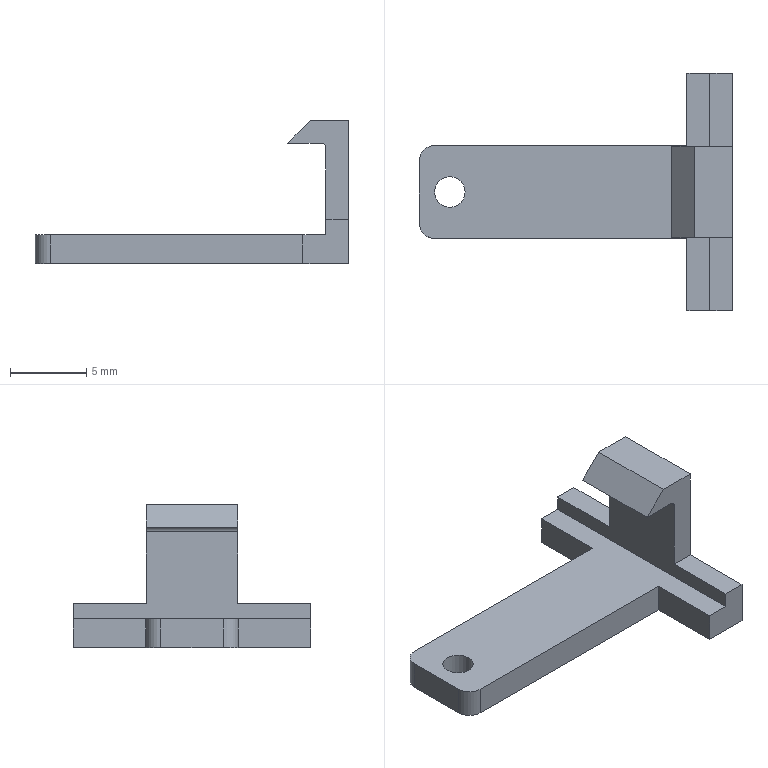Part | NX | features BREP 2, REPLACE_FACE 1, UNITE 1 | 1 solid | 22 faces | box 20.555 x 15.6 x 9.4 mm | volume 383.369 mm3 | plane 18 | cylinder 4 | commonest cylinder face diameters 2 x3 0.6 x1
STEP:
#1=CARTESIAN_POINT('',(-22.19,-197.607,1.));
#2=VERTEX_POINT('',#1);
#3=CARTESIAN_POINT('',(-23.19,-197.607,1.));
#4=DIRECTION('',(0.,0.,1.));
#5=DIRECTION('',(1.,0.,0.));
#6=AXIS2_PLACEMENT_3D('',#3,#4,#5);
#7=CIRCLE('',#6,1.);
#8=EDGE_CURVE('',#2,#2,#7,.T.);
#9=ORIENTED_EDGE('',*,*,#8,.T.);
#10=EDGE_LOOP('',(#9));
#11=FACE_BOUND('',#10,.T.);
#12=CARTESIAN_POINT('',(-22.19,-197.607,-0.9));
#13=VERTEX_POINT('',#12);
#14=CARTESIAN_POINT('',(-23.19,-197.607,-0.9));
#15=DIRECTION('',(0.,0.,1.));
#16=DIRECTION('',(1.,0.,0.));
#17=AXIS2_PLACEMENT_3D('',#14,#15,#16);
#18=CIRCLE('',#17,1.);
#19=EDGE_CURVE('',#13,#13,#18,.T.);
#20=ORIENTED_EDGE('',*,*,#19,.F.);
#21=EDGE_LOOP('',(#20));
#22=FACE_BOUND('',#21,.T.);
#23=CARTESIAN_POINT('',(-23.19,-197.607,-9.));
#24=DIRECTION('',(0.,0.,1.));
#25=DIRECTION('',(-1.,0.,0.));
#26=AXIS2_PLACEMENT_3D('',#23,#24,#25);
#27=CYLINDRICAL_SURFACE('',#26,1.);
#28=ADVANCED_FACE('',(#11,#22),#27,.F.);
#29=CARTESIAN_POINT('',(-4.635,-189.807,2.));
#30=VERTEX_POINT('',#29);
#31=CARTESIAN_POINT('',(-6.135,-189.807,2.));
#32=VERTEX_POINT('',#31);
#33=CARTESIAN_POINT('',(0.,-189.807,2.));
#34=DIRECTION('',(-1.,0.,0.));
#35=VECTOR('',#34,1000.);
#36=LINE('',#33,#35);
#37=EDGE_CURVE('',#30,#32,#36,.T.);
#38=ORIENTED_EDGE('',*,*,#37,.T.);
#39=CARTESIAN_POINT('',(-6.135,-194.607,2.));
#40=VERTEX_POINT('',#39);
#41=CARTESIAN_POINT('',(-6.135,-184.759,2.));
#42=DIRECTION('',(0.,1.,0.));
#43=VECTOR('',#42,1000.);
#44=LINE('',#41,#43);
#45=EDGE_CURVE('',#40,#32,#44,.T.);
#46=ORIENTED_EDGE('',*,*,#45,.F.);
#47=CARTESIAN_POINT('',(-4.635,-194.607,2.));
#48=VERTEX_POINT('',#47);
#49=CARTESIAN_POINT('',(-28.167,-194.607,2.));
#50=DIRECTION('',(1.,0.,0.));
#51=VECTOR('',#50,1000.);
#52=LINE('',#49,#51);
#53=EDGE_CURVE('',#40,#48,#52,.T.);
#54=ORIENTED_EDGE('',*,*,#53,.T.);
#55=CARTESIAN_POINT('',(-4.635,-200.607,2.));
#56=DIRECTION('',(0.,1.,0.));
#57=VECTOR('',#56,1000.);
#58=LINE('',#55,#57);
#59=EDGE_CURVE('',#48,#30,#58,.T.);
#60=ORIENTED_EDGE('',*,*,#59,.T.);
#61=EDGE_LOOP('',(#38,#46,#54,#60));
#62=FACE_BOUND('',#61,.T.);
#63=CARTESIAN_POINT('',(0.,0.,2.));
#64=DIRECTION('',(0.,0.,1.));
#65=DIRECTION('',(-1.,0.,0.));
#66=AXIS2_PLACEMENT_3D('',#63,#64,#65);
#67=PLANE('',#66);
#68=ADVANCED_FACE('',(#62),#67,.T.);
#69=CARTESIAN_POINT('',(-6.135,-200.607,2.));
#70=VERTEX_POINT('',#69);
#71=CARTESIAN_POINT('',(-6.135,-205.407,2.));
#72=VERTEX_POINT('',#71);
#73=CARTESIAN_POINT('',(-6.135,0.,2.));
#74=DIRECTION('',(0.,-1.,0.));
#75=VECTOR('',#74,1000.);
#76=LINE('',#73,#75);
#77=EDGE_CURVE('',#70,#72,#76,.T.);
#78=ORIENTED_EDGE('',*,*,#77,.T.);
#79=CARTESIAN_POINT('',(-4.635,-205.407,2.));
#80=VERTEX_POINT('',#79);
#81=CARTESIAN_POINT('',(0.,-205.407,2.));
#82=DIRECTION('',(1.,0.,0.));
#83=VECTOR('',#82,1000.);
#84=LINE('',#81,#83);
#85=EDGE_CURVE('',#72,#80,#84,.T.);
#86=ORIENTED_EDGE('',*,*,#85,.T.);
#87=CARTESIAN_POINT('',(-4.635,-200.607,2.));
#88=VERTEX_POINT('',#87);
#89=CARTESIAN_POINT('',(-4.635,-200.607,2.));
#90=DIRECTION('',(0.,1.,0.));
#91=VECTOR('',#90,1000.);
#92=LINE('',#89,#91);
#93=EDGE_CURVE('',#80,#88,#92,.T.);
#94=ORIENTED_EDGE('',*,*,#93,.T.);
#95=CARTESIAN_POINT('',(-28.167,-200.607,2.));
#96=DIRECTION('',(-1.,0.,0.));
#97=VECTOR('',#96,1000.);
#98=LINE('',#95,#97);
#99=EDGE_CURVE('',#88,#70,#98,.T.);
#100=ORIENTED_EDGE('',*,*,#99,.T.);
#101=EDGE_LOOP('',(#78,#86,#94,#100));
#102=FACE_BOUND('',#101,.T.);
#103=CARTESIAN_POINT('',(0.,0.,2.));
#104=DIRECTION('',(0.,0.,1.));
#105=DIRECTION('',(-1.,0.,0.));
#106=AXIS2_PLACEMENT_3D('',#103,#104,#105);
#107=PLANE('',#106);
#108=ADVANCED_FACE('',(#102),#107,.T.);
#109=ORIENTED_EDGE('',*,*,#85,.F.);
#110=CARTESIAN_POINT('',(-6.135,-205.407,1.));
#111=VERTEX_POINT('',#110);
#112=CARTESIAN_POINT('',(-6.135,-205.407,0.));
#113=DIRECTION('',(0.,0.,-1.));
#114=VECTOR('',#113,1000.);
#115=LINE('',#112,#114);
#116=EDGE_CURVE('',#72,#111,#115,.T.);
#117=ORIENTED_EDGE('',*,*,#116,.T.);
#118=CARTESIAN_POINT('',(-7.635,-205.407,1.));
#119=VERTEX_POINT('',#118);
#120=CARTESIAN_POINT('',(-4.635,-205.407,1.));
#121=DIRECTION('',(-1.,0.,0.));
#122=VECTOR('',#121,1000.);
#123=LINE('',#120,#122);
#124=EDGE_CURVE('',#111,#119,#123,.T.);
#125=ORIENTED_EDGE('',*,*,#124,.T.);
#126=CARTESIAN_POINT('',(-7.635,-205.407,-0.9));
#127=VERTEX_POINT('',#126);
#128=CARTESIAN_POINT('',(-7.635,-205.407,0.));
#129=DIRECTION('',(0.,0.,1.));
#130=VECTOR('',#129,1000.);
#131=LINE('',#128,#130);
#132=EDGE_CURVE('',#127,#119,#131,.T.);
#133=ORIENTED_EDGE('',*,*,#132,.F.);
#134=CARTESIAN_POINT('',(-4.635,-205.407,-0.9));
#135=VERTEX_POINT('',#134);
#136=CARTESIAN_POINT('',(0.,-205.407,-0.9));
#137=DIRECTION('',(1.,0.,0.));
#138=VECTOR('',#137,1000.);
#139=LINE('',#136,#138);
#140=EDGE_CURVE('',#127,#135,#139,.T.);
#141=ORIENTED_EDGE('',*,*,#140,.T.);
#142=CARTESIAN_POINT('',(-4.635,-205.407,2.));
#143=DIRECTION('',(0.,0.,1.));
#144=VECTOR('',#143,1000.);
#145=LINE('',#142,#144);
#146=EDGE_CURVE('',#135,#80,#145,.T.);
#147=ORIENTED_EDGE('',*,*,#146,.T.);
#148=EDGE_LOOP('',(#109,#117,#125,#133,#141,#147));
#149=FACE_BOUND('',#148,.T.);
#150=CARTESIAN_POINT('',(-4.635,-205.407,0.));
#151=DIRECTION('',(0.,-1.,0.));
#152=DIRECTION('',(0.,0.,1.));
#153=AXIS2_PLACEMENT_3D('',#150,#151,#152);
#154=PLANE('',#153);
#155=ADVANCED_FACE('',(#149),#154,.T.);
#156=ORIENTED_EDGE('',*,*,#132,.T.);
#157=CARTESIAN_POINT('',(-7.635,-200.657,1.));
#158=VERTEX_POINT('',#157);
#159=CARTESIAN_POINT('',(-7.635,0.,1.));
#160=DIRECTION('',(0.,-1.,0.));
#161=VECTOR('',#160,1000.);
#162=LINE('',#159,#161);
#163=EDGE_CURVE('',#158,#119,#162,.T.);
#164=ORIENTED_EDGE('',*,*,#163,.F.);
#165=CARTESIAN_POINT('',(-7.635,-200.657,-0.9));
#166=VERTEX_POINT('',#165);
#167=CARTESIAN_POINT('',(-7.635,-200.657,2.));
#168=DIRECTION('',(0.,0.,1.));
#169=VECTOR('',#168,1000.);
#170=LINE('',#167,#169);
#171=EDGE_CURVE('',#166,#158,#170,.T.);
#172=ORIENTED_EDGE('',*,*,#171,.F.);
#173=CARTESIAN_POINT('',(-7.635,0.,-0.9));
#174=DIRECTION('',(0.,-1.,0.));
#175=VECTOR('',#174,1000.);
#176=LINE('',#173,#175);
#177=EDGE_CURVE('',#166,#127,#176,.T.);
#178=ORIENTED_EDGE('',*,*,#177,.T.);
#179=EDGE_LOOP('',(#156,#164,#172,#178));
#180=FACE_BOUND('',#179,.T.);
#181=CARTESIAN_POINT('',(-7.635,-203.607,0.));
#182=DIRECTION('',(-1.,0.,0.));
#183=DIRECTION('',(0.,-1.,0.));
#184=AXIS2_PLACEMENT_3D('',#181,#182,#183);
#185=PLANE('',#184);
#186=ADVANCED_FACE('',(#180),#185,.T.);
#187=CARTESIAN_POINT('',(-7.635,-194.557,1.));
#188=VERTEX_POINT('',#187);
#189=CARTESIAN_POINT('',(-7.635,-189.807,1.));
#190=VERTEX_POINT('',#189);
#191=CARTESIAN_POINT('',(-7.635,-191.607,1.));
#192=DIRECTION('',(0.,1.,0.));
#193=VECTOR('',#192,1000.);
#194=LINE('',#191,#193);
#195=EDGE_CURVE('',#188,#190,#194,.T.);
#196=ORIENTED_EDGE('',*,*,#195,.T.);
#197=CARTESIAN_POINT('',(-7.635,-189.807,-0.9));
#198=VERTEX_POINT('',#197);
#199=CARTESIAN_POINT('',(-7.635,-189.807,0.));
#200=DIRECTION('',(0.,0.,1.));
#201=VECTOR('',#200,1000.);
#202=LINE('',#199,#201);
#203=EDGE_CURVE('',#198,#190,#202,.T.);
#204=ORIENTED_EDGE('',*,*,#203,.F.);
#205=CARTESIAN_POINT('',(-7.635,-194.557,-0.9));
#206=VERTEX_POINT('',#205);
#207=CARTESIAN_POINT('',(-7.635,0.,-0.9));
#208=DIRECTION('',(0.,-1.,0.));
#209=VECTOR('',#208,1000.);
#210=LINE('',#207,#209);
#211=EDGE_CURVE('',#198,#206,#210,.T.);
#212=ORIENTED_EDGE('',*,*,#211,.T.);
#213=CARTESIAN_POINT('',(-7.635,-194.557,0.));
#214=DIRECTION('',(0.,0.,1.));
#215=VECTOR('',#214,1000.);
#216=LINE('',#213,#215);
#217=EDGE_CURVE('',#206,#188,#216,.T.);
#218=ORIENTED_EDGE('',*,*,#217,.T.);
#219=EDGE_LOOP('',(#196,#204,#212,#218));
#220=FACE_BOUND('',#219,.T.);
#221=CARTESIAN_POINT('',(-7.635,-191.607,0.));
#222=DIRECTION('',(-1.,0.,0.));
#223=DIRECTION('',(0.,0.,-1.));
#224=AXIS2_PLACEMENT_3D('',#221,#222,#223);
#225=PLANE('',#224);
#226=ADVANCED_FACE('',(#220),#225,.T.);
#227=CARTESIAN_POINT('',(-6.135,-189.807,1.));
#228=VERTEX_POINT('',#227);
#229=CARTESIAN_POINT('',(-4.635,-189.807,1.));
#230=DIRECTION('',(1.,0.,0.));
#231=VECTOR('',#230,1000.);
#232=LINE('',#229,#231);
#233=EDGE_CURVE('',#190,#228,#232,.T.);
#234=ORIENTED_EDGE('',*,*,#233,.T.);
#235=CARTESIAN_POINT('',(-6.135,-189.807,0.));
#236=DIRECTION('',(0.,0.,1.));
#237=VECTOR('',#236,1000.);
#238=LINE('',#235,#237);
#239=EDGE_CURVE('',#228,#32,#238,.T.);
#240=ORIENTED_EDGE('',*,*,#239,.T.);
#241=ORIENTED_EDGE('',*,*,#37,.F.);
#242=CARTESIAN_POINT('',(-4.635,-189.807,-0.9));
#243=VERTEX_POINT('',#242);
#244=CARTESIAN_POINT('',(-4.635,-189.807,0.));
#245=DIRECTION('',(0.,0.,1.));
#246=VECTOR('',#245,1000.);
#247=LINE('',#244,#246);
#248=EDGE_CURVE('',#243,#30,#247,.T.);
#249=ORIENTED_EDGE('',*,*,#248,.F.);
#250=CARTESIAN_POINT('',(0.,-189.807,-0.9));
#251=DIRECTION('',(-1.,0.,0.));
#252=VECTOR('',#251,1000.);
#253=LINE('',#250,#252);
#254=EDGE_CURVE('',#243,#198,#253,.T.);
#255=ORIENTED_EDGE('',*,*,#254,.T.);
#256=ORIENTED_EDGE('',*,*,#203,.T.);
#257=EDGE_LOOP('',(#234,#240,#241,#249,#255,#256));
#258=FACE_BOUND('',#257,.T.);
#259=CARTESIAN_POINT('',(-4.635,-189.807,0.));
#260=DIRECTION('',(0.,1.,0.));
#261=DIRECTION('',(-1.,0.,0.));
#262=AXIS2_PLACEMENT_3D('',#259,#260,#261);
#263=PLANE('',#262);
#264=ADVANCED_FACE('',(#258),#263,.T.);
#265=CARTESIAN_POINT('',(-24.19,-194.557,-0.9));
#266=VERTEX_POINT('',#265);
#267=CARTESIAN_POINT('',(-4.635,-194.557,-0.9));
#268=DIRECTION('',(-1.,0.,0.));
#269=VECTOR('',#268,1000.);
#270=LINE('',#267,#269);
#271=EDGE_CURVE('',#206,#266,#270,.T.);
#272=ORIENTED_EDGE('',*,*,#271,.T.);
#273=CARTESIAN_POINT('',(-24.19,-194.557,1.));
#274=VERTEX_POINT('',#273);
#275=CARTESIAN_POINT('',(-24.19,-194.557,2.));
#276=DIRECTION('',(0.,0.,1.));
#277=VECTOR('',#276,1000.);
#278=LINE('',#275,#277);
#279=EDGE_CURVE('',#266,#274,#278,.T.);
#280=ORIENTED_EDGE('',*,*,#279,.T.);
#281=CARTESIAN_POINT('',(-4.635,-194.557,1.));
#282=DIRECTION('',(-1.,0.,0.));
#283=VECTOR('',#282,1000.);
#284=LINE('',#281,#283);
#285=EDGE_CURVE('',#188,#274,#284,.T.);
#286=ORIENTED_EDGE('',*,*,#285,.F.);
#287=ORIENTED_EDGE('',*,*,#217,.F.);
#288=EDGE_LOOP('',(#272,#280,#286,#287));
#289=FACE_BOUND('',#288,.T.);
#290=CARTESIAN_POINT('',(-4.635,-194.557,2.));
#291=DIRECTION('',(0.,-1.,0.));
#292=DIRECTION('',(0.,0.,1.));
#293=AXIS2_PLACEMENT_3D('',#290,#291,#292);
#294=PLANE('',#293);
#295=ADVANCED_FACE('',(#289),#294,.F.);
#296=CARTESIAN_POINT('',(-24.19,-200.657,1.));
#297=VERTEX_POINT('',#296);
#298=CARTESIAN_POINT('',(-4.635,-200.657,1.));
#299=DIRECTION('',(1.,0.,0.));
#300=VECTOR('',#299,1000.);
#301=LINE('',#298,#300);
#302=EDGE_CURVE('',#297,#158,#301,.T.);
#303=ORIENTED_EDGE('',*,*,#302,.F.);
#304=CARTESIAN_POINT('',(-24.19,-200.657,-0.9));
#305=VERTEX_POINT('',#304);
#306=CARTESIAN_POINT('',(-24.19,-200.657,2.));
#307=DIRECTION('',(0.,0.,-1.));
#308=VECTOR('',#307,1000.);
#309=LINE('',#306,#308);
#310=EDGE_CURVE('',#297,#305,#309,.T.);
#311=ORIENTED_EDGE('',*,*,#310,.T.);
#312=CARTESIAN_POINT('',(-4.635,-200.657,-0.9));
#313=DIRECTION('',(1.,0.,0.));
#314=VECTOR('',#313,1000.);
#315=LINE('',#312,#314);
#316=EDGE_CURVE('',#305,#166,#315,.T.);
#317=ORIENTED_EDGE('',*,*,#316,.T.);
#318=ORIENTED_EDGE('',*,*,#171,.T.);
#319=EDGE_LOOP('',(#303,#311,#317,#318));
#320=FACE_BOUND('',#319,.T.);
#321=CARTESIAN_POINT('',(-4.635,-200.657,2.));
#322=DIRECTION('',(0.,1.,0.));
#323=DIRECTION('',(-1.,0.,0.));
#324=AXIS2_PLACEMENT_3D('',#321,#322,#323);
#325=PLANE('',#324);
#326=ADVANCED_FACE('',(#320),#325,.F.);
#327=CARTESIAN_POINT('',(-25.19,-195.557,-0.9));
#328=VERTEX_POINT('',#327);
#329=CARTESIAN_POINT('',(-25.19,-199.657,-0.9));
#330=VERTEX_POINT('',#329);
#331=CARTESIAN_POINT('',(-25.19,-200.607,-0.9));
#332=DIRECTION('',(0.,-1.,0.));
#333=VECTOR('',#332,1000.);
#334=LINE('',#331,#333);
#335=EDGE_CURVE('',#328,#330,#334,.T.);
#336=ORIENTED_EDGE('',*,*,#335,.T.);
#337=CARTESIAN_POINT('',(-25.19,-199.657,1.));
#338=VERTEX_POINT('',#337);
#339=CARTESIAN_POINT('',(-25.19,-199.657,2.));
#340=DIRECTION('',(0.,0.,1.));
#341=VECTOR('',#340,1000.);
#342=LINE('',#339,#341);
#343=EDGE_CURVE('',#330,#338,#342,.T.);
#344=ORIENTED_EDGE('',*,*,#343,.T.);
#345=CARTESIAN_POINT('',(-25.19,-195.557,1.));
#346=VERTEX_POINT('',#345);
#347=CARTESIAN_POINT('',(-25.19,-194.607,1.));
#348=DIRECTION('',(0.,-1.,0.));
#349=VECTOR('',#348,1000.);
#350=LINE('',#347,#349);
#351=EDGE_CURVE('',#346,#338,#350,.T.);
#352=ORIENTED_EDGE('',*,*,#351,.F.);
#353=CARTESIAN_POINT('',(-25.19,-195.557,2.));
#354=DIRECTION('',(0.,0.,-1.));
#355=VECTOR('',#354,1000.);
#356=LINE('',#353,#355);
#357=EDGE_CURVE('',#346,#328,#356,.T.);
#358=ORIENTED_EDGE('',*,*,#357,.T.);
#359=EDGE_LOOP('',(#336,#344,#352,#358));
#360=FACE_BOUND('',#359,.T.);
#361=CARTESIAN_POINT('',(-25.19,-200.607,2.));
#362=DIRECTION('',(1.,0.,0.));
#363=DIRECTION('',(0.,-1.,0.));
#364=AXIS2_PLACEMENT_3D('',#361,#362,#363);
#365=PLANE('',#364);
#366=ADVANCED_FACE('',(#360),#365,.F.);
#367=CARTESIAN_POINT('',(-4.635,-194.607,8.5));
#368=VERTEX_POINT('',#367);
#369=CARTESIAN_POINT('',(-4.635,-194.607,2.));
#370=DIRECTION('',(0.,0.,-1.));
#371=VECTOR('',#370,1000.);
#372=LINE('',#369,#371);
#373=EDGE_CURVE('',#368,#48,#372,.T.);
#374=ORIENTED_EDGE('',*,*,#373,.F.);
#375=CARTESIAN_POINT('',(-4.635,-200.607,8.5));
#376=VERTEX_POINT('',#375);
#377=CARTESIAN_POINT('',(-4.635,-200.607,8.5));
#378=DIRECTION('',(0.,-1.,0.));
#379=VECTOR('',#378,1000.);
#380=LINE('',#377,#379);
#381=EDGE_CURVE('',#368,#376,#380,.T.);
#382=ORIENTED_EDGE('',*,*,#381,.T.);
#383=CARTESIAN_POINT('',(-4.635,-200.607,2.));
#384=DIRECTION('',(0.,0.,1.));
#385=VECTOR('',#384,1000.);
#386=LINE('',#383,#385);
#387=EDGE_CURVE('',#88,#376,#386,.T.);
#388=ORIENTED_EDGE('',*,*,#387,.F.);
#389=ORIENTED_EDGE('',*,*,#93,.F.);
#390=ORIENTED_EDGE('',*,*,#146,.F.);
#391=CARTESIAN_POINT('',(-4.635,-200.607,-0.9));
#392=DIRECTION('',(0.,1.,0.));
#393=VECTOR('',#392,1000.);
#394=LINE('',#391,#393);
#395=EDGE_CURVE('',#135,#243,#394,.T.);
#396=ORIENTED_EDGE('',*,*,#395,.T.);
#397=ORIENTED_EDGE('',*,*,#248,.T.);
#398=ORIENTED_EDGE('',*,*,#59,.F.);
#399=EDGE_LOOP('',(#374,#382,#388,#389,#390,#396,#397,#398));
#400=FACE_BOUND('',#399,.T.);
#401=CARTESIAN_POINT('',(-4.635,-200.607,2.));
#402=DIRECTION('',(-1.,0.,0.));
#403=DIRECTION('',(0.,0.,-1.));
#404=AXIS2_PLACEMENT_3D('',#401,#402,#403);
#405=PLANE('',#404);
#406=ADVANCED_FACE('',(#400),#405,.F.);
#407=CARTESIAN_POINT('',(-6.135,-200.607,6.7));
#408=VERTEX_POINT('',#407);
#409=CARTESIAN_POINT('',(-6.135,-200.607,7.));
#410=DIRECTION('',(0.,0.,1.));
#411=VECTOR('',#410,1000.);
#412=LINE('',#409,#411);
#413=EDGE_CURVE('',#70,#408,#412,.T.);
#414=ORIENTED_EDGE('',*,*,#413,.T.);
#415=CARTESIAN_POINT('',(-6.135,-194.607,6.7));
#416=VERTEX_POINT('',#415);
#417=CARTESIAN_POINT('',(-6.135,-184.759,6.7));
#418=DIRECTION('',(0.,1.,0.));
#419=VECTOR('',#418,1000.);
#420=LINE('',#417,#419);
#421=EDGE_CURVE('',#408,#416,#420,.T.);
#422=ORIENTED_EDGE('',*,*,#421,.T.);
#423=CARTESIAN_POINT('',(-6.135,-194.607,7.));
#424=DIRECTION('',(0.,0.,-1.));
#425=VECTOR('',#424,1000.);
#426=LINE('',#423,#425);
#427=EDGE_CURVE('',#416,#40,#426,.T.);
#428=ORIENTED_EDGE('',*,*,#427,.T.);
#429=ORIENTED_EDGE('',*,*,#45,.T.);
#430=ORIENTED_EDGE('',*,*,#239,.F.);
#431=CARTESIAN_POINT('',(-6.135,-200.607,1.));
#432=DIRECTION('',(0.,1.,0.));
#433=VECTOR('',#432,1000.);
#434=LINE('',#431,#433);
#435=EDGE_CURVE('',#111,#228,#434,.T.);
#436=ORIENTED_EDGE('',*,*,#435,.F.);
#437=ORIENTED_EDGE('',*,*,#116,.F.);
#438=ORIENTED_EDGE('',*,*,#77,.F.);
#439=EDGE_LOOP('',(#414,#422,#428,#429,#430,#436,#437,#438));
#440=FACE_BOUND('',#439,.T.);
#441=CARTESIAN_POINT('',(-6.135,-184.759,7.));
#442=DIRECTION('',(-1.,0.,0.));
#443=DIRECTION('',(0.,0.,-1.));
#444=AXIS2_PLACEMENT_3D('',#441,#442,#443);
#445=PLANE('',#444);
#446=ADVANCED_FACE('',(#440),#445,.T.);
#447=CARTESIAN_POINT('',(-7.135,-194.607,8.5));
#448=VERTEX_POINT('',#447);
#449=CARTESIAN_POINT('',(-8.635,-194.607,7.));
#450=VERTEX_POINT('',#449);
#451=CARTESIAN_POINT('',(-4.635,-194.607,11.));
#452=DIRECTION('',(-0.7071,0.,-0.7071));
#453=VECTOR('',#452,1000.);
#454=LINE('',#451,#453);
#455=EDGE_CURVE('',#448,#450,#454,.T.);
#456=ORIENTED_EDGE('',*,*,#455,.T.);
#457=CARTESIAN_POINT('',(-8.635,-200.607,7.));
#458=VERTEX_POINT('',#457);
#459=CARTESIAN_POINT('',(-8.635,-184.759,7.));
#460=DIRECTION('',(0.,-1.,0.));
#461=VECTOR('',#460,1000.);
#462=LINE('',#459,#461);
#463=EDGE_CURVE('',#450,#458,#462,.T.);
#464=ORIENTED_EDGE('',*,*,#463,.T.);
#465=CARTESIAN_POINT('',(-7.135,-200.607,8.5));
#466=VERTEX_POINT('',#465);
#467=CARTESIAN_POINT('',(-4.635,-200.607,11.));
#468=DIRECTION('',(0.7071,0.,0.7071));
#469=VECTOR('',#468,1000.);
#470=LINE('',#467,#469);
#471=EDGE_CURVE('',#458,#466,#470,.T.);
#472=ORIENTED_EDGE('',*,*,#471,.T.);
#473=CARTESIAN_POINT('',(-7.135,-184.759,8.5));
#474=DIRECTION('',(0.,-1.,0.));
#475=VECTOR('',#474,1000.);
#476=LINE('',#473,#475);
#477=EDGE_CURVE('',#448,#466,#476,.T.);
#478=ORIENTED_EDGE('',*,*,#477,.F.);
#479=EDGE_LOOP('',(#456,#464,#472,#478));
#480=FACE_BOUND('',#479,.T.);
#481=CARTESIAN_POINT('',(-4.635,-184.759,11.));
#482=DIRECTION('',(-0.7071,0.,0.7071));
#483=DIRECTION('',(0.,-1.,0.));
#484=AXIS2_PLACEMENT_3D('',#481,#482,#483);
#485=PLANE('',#484);
#486=ADVANCED_FACE('',(#480),#485,.T.);
#487=ORIENTED_EDGE('',*,*,#316,.F.);
#488=CARTESIAN_POINT('',(-24.19,-199.657,-0.9));
#489=DIRECTION('',(0.,0.,-1.));
#490=DIRECTION('',(1.,0.,0.));
#491=AXIS2_PLACEMENT_3D('',#488,#489,#490);
#492=CIRCLE('',#491,1.);
#493=EDGE_CURVE('',#305,#330,#492,.T.);
#494=ORIENTED_EDGE('',*,*,#493,.T.);
#495=ORIENTED_EDGE('',*,*,#335,.F.);
#496=CARTESIAN_POINT('',(-24.19,-195.557,-0.9));
#497=DIRECTION('',(0.,0.,-1.));
#498=DIRECTION('',(1.,0.,0.));
#499=AXIS2_PLACEMENT_3D('',#496,#497,#498);
#500=CIRCLE('',#499,1.);
#501=EDGE_CURVE('',#328,#266,#500,.T.);
#502=ORIENTED_EDGE('',*,*,#501,.T.);
#503=ORIENTED_EDGE('',*,*,#271,.F.);
#504=ORIENTED_EDGE('',*,*,#211,.F.);
#505=ORIENTED_EDGE('',*,*,#254,.F.);
#506=ORIENTED_EDGE('',*,*,#395,.F.);
#507=ORIENTED_EDGE('',*,*,#140,.F.);
#508=ORIENTED_EDGE('',*,*,#177,.F.);
#509=EDGE_LOOP('',(#487,#494,#495,#502,#503,#504,#505,#506,#507,#508));
#510=FACE_BOUND('',#509,.T.);
#511=ORIENTED_EDGE('',*,*,#19,.T.);
#512=EDGE_LOOP('',(#511));
#513=FACE_BOUND('',#512,.T.);
#514=CARTESIAN_POINT('',(0.,0.,-0.9));
#515=DIRECTION('',(0.,0.,1.));
#516=DIRECTION('',(-1.,0.,0.));
#517=AXIS2_PLACEMENT_3D('',#514,#515,#516);
#518=PLANE('',#517);
#519=ADVANCED_FACE('',(#510,#513),#518,.F.);
#520=CARTESIAN_POINT('',(-6.435,-194.607,7.));
#521=VERTEX_POINT('',#520);
#522=CARTESIAN_POINT('',(-8.635,-194.607,7.));
#523=DIRECTION('',(1.,0.,0.));
#524=VECTOR('',#523,1000.);
#525=LINE('',#522,#524);
#526=EDGE_CURVE('',#450,#521,#525,.T.);
#527=ORIENTED_EDGE('',*,*,#526,.F.);
#528=ORIENTED_EDGE('',*,*,#455,.F.);
#529=CARTESIAN_POINT('',(-28.167,-194.607,8.5));
#530=DIRECTION('',(-1.,0.,0.));
#531=VECTOR('',#530,1000.);
#532=LINE('',#529,#531);
#533=EDGE_CURVE('',#368,#448,#532,.T.);
#534=ORIENTED_EDGE('',*,*,#533,.F.);
#535=ORIENTED_EDGE('',*,*,#373,.T.);
#536=ORIENTED_EDGE('',*,*,#53,.F.);
#537=ORIENTED_EDGE('',*,*,#427,.F.);
#538=CARTESIAN_POINT('',(-6.435,-194.607,6.7));
#539=DIRECTION('',(0.,1.,0.));
#540=DIRECTION('',(0.,0.,1.));
#541=AXIS2_PLACEMENT_3D('',#538,#539,#540);
#542=CIRCLE('',#541,0.3);
#543=EDGE_CURVE('',#416,#521,#542,.F.);
#544=ORIENTED_EDGE('',*,*,#543,.T.);
#545=EDGE_LOOP('',(#527,#528,#534,#535,#536,#537,#544));
#546=FACE_BOUND('',#545,.T.);
#547=CARTESIAN_POINT('',(-28.167,-194.607,34.));
#548=DIRECTION('',(0.,1.,0.));
#549=DIRECTION('',(-1.,0.,0.));
#550=AXIS2_PLACEMENT_3D('',#547,#548,#549);
#551=PLANE('',#550);
#552=ADVANCED_FACE('',(#546),#551,.T.);
#553=ORIENTED_EDGE('',*,*,#471,.F.);
#554=CARTESIAN_POINT('',(-6.435,-200.607,7.));
#555=VERTEX_POINT('',#554);
#556=CARTESIAN_POINT('',(-28.167,-200.607,7.));
#557=DIRECTION('',(1.,0.,0.));
#558=VECTOR('',#557,1000.);
#559=LINE('',#556,#558);
#560=EDGE_CURVE('',#458,#555,#559,.T.);
#561=ORIENTED_EDGE('',*,*,#560,.T.);
#562=CARTESIAN_POINT('',(-6.435,-200.607,6.7));
#563=DIRECTION('',(0.,-1.,0.));
#564=DIRECTION('',(0.,0.,-1.));
#565=AXIS2_PLACEMENT_3D('',#562,#563,#564);
#566=CIRCLE('',#565,0.3);
#567=EDGE_CURVE('',#555,#408,#566,.F.);
#568=ORIENTED_EDGE('',*,*,#567,.T.);
#569=ORIENTED_EDGE('',*,*,#413,.F.);
#570=ORIENTED_EDGE('',*,*,#99,.F.);
#571=ORIENTED_EDGE('',*,*,#387,.T.);
#572=CARTESIAN_POINT('',(-28.167,-200.607,8.5));
#573=DIRECTION('',(1.,0.,0.));
#574=VECTOR('',#573,1000.);
#575=LINE('',#572,#574);
#576=EDGE_CURVE('',#466,#376,#575,.T.);
#577=ORIENTED_EDGE('',*,*,#576,.F.);
#578=EDGE_LOOP('',(#553,#561,#568,#569,#570,#571,#577));
#579=FACE_BOUND('',#578,.T.);
#580=CARTESIAN_POINT('',(-28.167,-200.607,34.));
#581=DIRECTION('',(0.,-1.,0.));
#582=DIRECTION('',(0.,0.,1.));
#583=AXIS2_PLACEMENT_3D('',#580,#581,#582);
#584=PLANE('',#583);
#585=ADVANCED_FACE('',(#579),#584,.T.);
#586=ORIENTED_EDGE('',*,*,#533,.T.);
#587=ORIENTED_EDGE('',*,*,#477,.T.);
#588=ORIENTED_EDGE('',*,*,#576,.T.);
#589=ORIENTED_EDGE('',*,*,#381,.F.);
#590=EDGE_LOOP('',(#586,#587,#588,#589));
#591=FACE_BOUND('',#590,.T.);
#592=CARTESIAN_POINT('',(-9.497,-190.607,8.5));
#593=DIRECTION('',(0.,0.,-1.));
#594=DIRECTION('',(0.,1.,0.));
#595=AXIS2_PLACEMENT_3D('',#592,#593,#594);
#596=PLANE('',#595);
#597=ADVANCED_FACE('',(#591),#596,.F.);
#598=ORIENTED_EDGE('',*,*,#351,.T.);
#599=CARTESIAN_POINT('',(-24.19,-199.657,1.));
#600=DIRECTION('',(0.,0.,1.));
#601=DIRECTION('',(1.,0.,0.));
#602=AXIS2_PLACEMENT_3D('',#599,#600,#601);
#603=CIRCLE('',#602,1.);
#604=EDGE_CURVE('',#338,#297,#603,.T.);
#605=ORIENTED_EDGE('',*,*,#604,.T.);
#606=ORIENTED_EDGE('',*,*,#302,.T.);
#607=ORIENTED_EDGE('',*,*,#163,.T.);
#608=ORIENTED_EDGE('',*,*,#124,.F.);
#609=ORIENTED_EDGE('',*,*,#435,.T.);
#610=ORIENTED_EDGE('',*,*,#233,.F.);
#611=ORIENTED_EDGE('',*,*,#195,.F.);
#612=ORIENTED_EDGE('',*,*,#285,.T.);
#613=CARTESIAN_POINT('',(-24.19,-195.557,1.));
#614=DIRECTION('',(0.,0.,1.));
#615=DIRECTION('',(1.,0.,0.));
#616=AXIS2_PLACEMENT_3D('',#613,#614,#615);
#617=CIRCLE('',#616,1.);
#618=EDGE_CURVE('',#274,#346,#617,.T.);
#619=ORIENTED_EDGE('',*,*,#618,.T.);
#620=EDGE_LOOP('',(#598,#605,#606,#607,#608,#609,#610,#611,#612,#619));
#621=FACE_BOUND('',#620,.T.);
#622=ORIENTED_EDGE('',*,*,#8,.F.);
#623=EDGE_LOOP('',(#622));
#624=FACE_BOUND('',#623,.T.);
#625=CARTESIAN_POINT('',(0.,0.,1.));
#626=DIRECTION('',(0.,0.,1.));
#627=DIRECTION('',(-1.,0.,0.));
#628=AXIS2_PLACEMENT_3D('',#625,#626,#627);
#629=PLANE('',#628);
#630=ADVANCED_FACE('',(#621,#624),#629,.T.);
#631=ORIENTED_EDGE('',*,*,#604,.F.);
#632=ORIENTED_EDGE('',*,*,#343,.F.);
#633=ORIENTED_EDGE('',*,*,#493,.F.);
#634=ORIENTED_EDGE('',*,*,#310,.F.);
#635=EDGE_LOOP('',(#631,#632,#633,#634));
#636=FACE_BOUND('',#635,.T.);
#637=CARTESIAN_POINT('',(-24.19,-199.657,2.));
#638=DIRECTION('',(0.,0.,-1.));
#639=DIRECTION('',(1.,0.,0.));
#640=AXIS2_PLACEMENT_3D('',#637,#638,#639);
#641=CYLINDRICAL_SURFACE('',#640,1.);
#642=ADVANCED_FACE('',(#636),#641,.T.);
#643=ORIENTED_EDGE('',*,*,#618,.F.);
#644=ORIENTED_EDGE('',*,*,#279,.F.);
#645=ORIENTED_EDGE('',*,*,#501,.F.);
#646=ORIENTED_EDGE('',*,*,#357,.F.);
#647=EDGE_LOOP('',(#643,#644,#645,#646));
#648=FACE_BOUND('',#647,.T.);
#649=CARTESIAN_POINT('',(-24.19,-195.557,2.));
#650=DIRECTION('',(0.,0.,-1.));
#651=DIRECTION('',(1.,0.,0.));
#652=AXIS2_PLACEMENT_3D('',#649,#650,#651);
#653=CYLINDRICAL_SURFACE('',#652,1.);
#654=ADVANCED_FACE('',(#648),#653,.T.);
#655=ORIENTED_EDGE('',*,*,#560,.F.);
#656=ORIENTED_EDGE('',*,*,#463,.F.);
#657=ORIENTED_EDGE('',*,*,#526,.T.);
#658=CARTESIAN_POINT('',(-6.435,-184.759,7.));
#659=DIRECTION('',(0.,1.,0.));
#660=VECTOR('',#659,1000.);
#661=LINE('',#658,#660);
#662=EDGE_CURVE('',#521,#555,#661,.F.);
#663=ORIENTED_EDGE('',*,*,#662,.T.);
#664=EDGE_LOOP('',(#655,#656,#657,#663));
#665=FACE_BOUND('',#664,.T.);
#666=CARTESIAN_POINT('',(-8.635,-184.759,7.));
#667=DIRECTION('',(0.,0.,-1.));
#668=DIRECTION('',(0.,1.,0.));
#669=AXIS2_PLACEMENT_3D('',#666,#667,#668);
#670=PLANE('',#669);
#671=ADVANCED_FACE('',(#665),#670,.T.);
#672=ORIENTED_EDGE('',*,*,#543,.F.);
#673=ORIENTED_EDGE('',*,*,#421,.F.);
#674=ORIENTED_EDGE('',*,*,#567,.F.);
#675=ORIENTED_EDGE('',*,*,#662,.F.);
#676=EDGE_LOOP('',(#672,#673,#674,#675));
#677=FACE_BOUND('',#676,.T.);
#678=CARTESIAN_POINT('',(-6.435,-184.759,6.7));
#679=DIRECTION('',(0.,-1.,0.));
#680=DIRECTION('',(0.,0.,-1.));
#681=AXIS2_PLACEMENT_3D('',#678,#679,#680);
#682=CYLINDRICAL_SURFACE('',#681,0.3);
#683=ADVANCED_FACE('',(#677),#682,.F.);
#684=CLOSED_SHELL('',(#28,#68,#108,#155,#186,#226,#264,#295,#326,#366,#406,#446,#486,#519,#552,#585,#597,#630,#642,#654,#671,#683));
#685=MANIFOLD_SOLID_BREP('',#684);
#686=(LENGTH_UNIT()NAMED_UNIT(*)SI_UNIT(.MILLI.,.METRE.));
#687=UNCERTAINTY_MEASURE_WITH_UNIT(LENGTH_MEASURE(0.00001),#686,'','');
#688=(NAMED_UNIT(*)PLANE_ANGLE_UNIT()SI_UNIT($,.RADIAN.));
#689=(NAMED_UNIT(*)SI_UNIT($,.STERADIAN.)SOLID_ANGLE_UNIT());
#690=(GEOMETRIC_REPRESENTATION_CONTEXT(3)GLOBAL_UNCERTAINTY_ASSIGNED_CONTEXT((#687))GLOBAL_UNIT_ASSIGNED_CONTEXT((#686,#688,#689))REPRESENTATION_CONTEXT('',''));
#691=ADVANCED_BREP_SHAPE_REPRESENTATION('',(#685),#690);